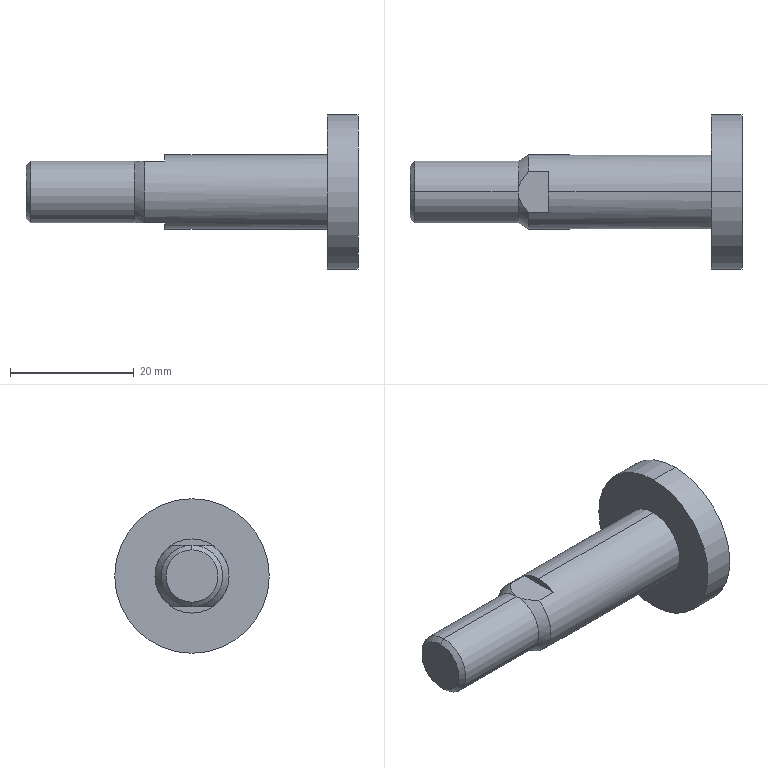Part | SolidWorks | features RefAxis 6, 3DProfileFeature 2, ICE 1, Revolution 1 | 1 solid | 17 faces | box 53.75 x 25 x 25 mm | volume 7288 mm3 | plane 7 | cylinder 6 | cone 4 | commonest cylinder face diameters 10 x2 12 x2 25 x2
STEP:
#1=CARTESIAN_POINT('',(31.25,0.,12.5));
#2=VERTEX_POINT('',#1);
#3=CARTESIAN_POINT('',(31.25,0.,-12.5));
#4=VERTEX_POINT('',#3);
#5=CARTESIAN_POINT('',(31.25,0.,0.));
#6=DIRECTION('',(-1.,0.,0.));
#7=DIRECTION('',(0.,0.,1.));
#8=AXIS2_PLACEMENT_3D('',#5,#6,#7);
#9=CIRCLE('',#8,12.5);
#10=EDGE_CURVE('',#2,#4,#9,.T.);
#11=ORIENTED_EDGE('',*,*,#10,.T.);
#12=CARTESIAN_POINT('',(26.25,0.,-12.5));
#13=VERTEX_POINT('',#12);
#14=CARTESIAN_POINT('',(31.25,0.,-12.5));
#15=DIRECTION('',(-1.,0.,0.));
#16=VECTOR('',#15,1000.);
#17=LINE('',#14,#16);
#18=EDGE_CURVE('',#4,#13,#17,.T.);
#19=ORIENTED_EDGE('',*,*,#18,.T.);
#20=CARTESIAN_POINT('',(26.25,0.,12.5));
#21=VERTEX_POINT('',#20);
#22=CARTESIAN_POINT('',(26.25,0.,0.));
#23=DIRECTION('',(-1.,0.,0.));
#24=DIRECTION('',(0.,0.,1.));
#25=AXIS2_PLACEMENT_3D('',#22,#23,#24);
#26=CIRCLE('',#25,12.5);
#27=EDGE_CURVE('',#21,#13,#26,.T.);
#28=ORIENTED_EDGE('',*,*,#27,.F.);
#29=CARTESIAN_POINT('',(31.25,0.,12.5));
#30=DIRECTION('',(-1.,0.,0.));
#31=VECTOR('',#30,1000.);
#32=LINE('',#29,#31);
#33=EDGE_CURVE('',#2,#21,#32,.T.);
#34=ORIENTED_EDGE('',*,*,#33,.F.);
#35=EDGE_LOOP('',(#11,#19,#28,#34));
#36=FACE_OUTER_BOUND('',#35,.T.);
#37=CARTESIAN_POINT('',(31.25,0.,0.));
#38=DIRECTION('',(-1.,0.,0.));
#39=DIRECTION('',(0.,0.,1.));
#40=AXIS2_PLACEMENT_3D('',#37,#38,#39);
#41=CYLINDRICAL_SURFACE('',#40,12.5);
#42=ADVANCED_FACE('',(#36),#41,.T.);
#43=CARTESIAN_POINT('',(-5.,0.,5.));
#44=VERTEX_POINT('',#43);
#45=CARTESIAN_POINT('',(-5.,0.,-5.));
#46=VERTEX_POINT('',#45);
#47=CARTESIAN_POINT('',(-5.,0.,0.));
#48=DIRECTION('',(-1.,0.,0.));
#49=DIRECTION('',(0.,0.,1.));
#50=AXIS2_PLACEMENT_3D('',#47,#48,#49);
#51=CIRCLE('',#50,5.);
#52=EDGE_CURVE('',#44,#46,#51,.T.);
#53=ORIENTED_EDGE('',*,*,#52,.T.);
#54=CARTESIAN_POINT('',(-21.733,0.,-5.));
#55=VERTEX_POINT('',#54);
#56=CARTESIAN_POINT('',(31.25,0.,-5.));
#57=DIRECTION('',(-1.,0.,0.));
#58=VECTOR('',#57,1000.);
#59=LINE('',#56,#58);
#60=EDGE_CURVE('',#46,#55,#59,.T.);
#61=ORIENTED_EDGE('',*,*,#60,.T.);
#62=CARTESIAN_POINT('',(-21.733,0.,5.));
#63=VERTEX_POINT('',#62);
#64=CARTESIAN_POINT('',(-21.733,0.,0.));
#65=DIRECTION('',(-1.,0.,0.));
#66=DIRECTION('',(0.,0.,1.));
#67=AXIS2_PLACEMENT_3D('',#64,#65,#66);
#68=CIRCLE('',#67,5.);
#69=EDGE_CURVE('',#63,#55,#68,.T.);
#70=ORIENTED_EDGE('',*,*,#69,.F.);
#71=CARTESIAN_POINT('',(31.25,0.,5.));
#72=DIRECTION('',(-1.,0.,0.));
#73=VECTOR('',#72,1000.);
#74=LINE('',#71,#73);
#75=EDGE_CURVE('',#44,#63,#74,.T.);
#76=ORIENTED_EDGE('',*,*,#75,.F.);
#77=EDGE_LOOP('',(#53,#61,#70,#76));
#78=FACE_OUTER_BOUND('',#77,.T.);
#79=CARTESIAN_POINT('',(31.25,0.,0.));
#80=DIRECTION('',(-1.,0.,0.));
#81=DIRECTION('',(0.,0.,1.));
#82=AXIS2_PLACEMENT_3D('',#79,#80,#81);
#83=CYLINDRICAL_SURFACE('',#82,5.);
#84=ADVANCED_FACE('',(#78),#83,.T.);
#85=CARTESIAN_POINT('',(-22.5,0.,4.233));
#86=VERTEX_POINT('',#85);
#87=CARTESIAN_POINT('',(-22.5,0.,-4.233));
#88=VERTEX_POINT('',#87);
#89=CARTESIAN_POINT('',(-22.5,0.,0.));
#90=DIRECTION('',(-1.,0.,0.));
#91=DIRECTION('',(0.,0.,1.));
#92=AXIS2_PLACEMENT_3D('',#89,#90,#91);
#93=CIRCLE('',#92,4.233);
#94=EDGE_CURVE('',#86,#88,#93,.T.);
#95=ORIENTED_EDGE('',*,*,#94,.F.);
#96=CARTESIAN_POINT('',(-21.733,0.,5.));
#97=DIRECTION('',(0.7071,0.,0.7071));
#98=VECTOR('',#97,1000.);
#99=LINE('',#96,#98);
#100=EDGE_CURVE('',#86,#63,#99,.T.);
#101=ORIENTED_EDGE('',*,*,#100,.T.);
#102=ORIENTED_EDGE('',*,*,#69,.T.);
#103=CARTESIAN_POINT('',(-21.733,0.,-5.));
#104=DIRECTION('',(0.7071,0.,-0.7071));
#105=VECTOR('',#104,1000.);
#106=LINE('',#103,#105);
#107=EDGE_CURVE('',#88,#55,#106,.T.);
#108=ORIENTED_EDGE('',*,*,#107,.F.);
#109=EDGE_LOOP('',(#95,#101,#102,#108));
#110=FACE_OUTER_BOUND('',#109,.T.);
#111=CARTESIAN_POINT('',(-21.733,0.,0.));
#112=DIRECTION('',(1.,0.,0.));
#113=DIRECTION('',(0.,0.,-1.));
#114=AXIS2_PLACEMENT_3D('',#111,#112,#113);
#115=CONICAL_SURFACE('',#114,5.,0.7854);
#116=ADVANCED_FACE('',(#110),#115,.T.);
#117=CARTESIAN_POINT('',(26.25,0.,6.));
#118=VERTEX_POINT('',#117);
#119=CARTESIAN_POINT('',(26.25,0.,-6.));
#120=VERTEX_POINT('',#119);
#121=CARTESIAN_POINT('',(26.25,0.,0.));
#122=DIRECTION('',(-1.,0.,0.));
#123=DIRECTION('',(0.,0.,1.));
#124=AXIS2_PLACEMENT_3D('',#121,#122,#123);
#125=CIRCLE('',#124,6.);
#126=EDGE_CURVE('',#118,#120,#125,.T.);
#127=ORIENTED_EDGE('',*,*,#126,.T.);
#128=CARTESIAN_POINT('',(0.,0.,-6.));
#129=VERTEX_POINT('',#128);
#130=CARTESIAN_POINT('',(31.25,0.,-6.));
#131=DIRECTION('',(-1.,0.,0.));
#132=VECTOR('',#131,1000.);
#133=LINE('',#130,#132);
#134=EDGE_CURVE('',#120,#129,#133,.T.);
#135=ORIENTED_EDGE('',*,*,#134,.T.);
#136=CARTESIAN_POINT('',(0.,3.317,-5.));
#137=VERTEX_POINT('',#136);
#138=CARTESIAN_POINT('',(0.,0.,0.));
#139=DIRECTION('',(1.,0.,0.));
#140=DIRECTION('',(0.,0.,-1.));
#141=AXIS2_PLACEMENT_3D('',#138,#139,#140);
#142=CIRCLE('',#141,6.);
#143=EDGE_CURVE('',#129,#137,#142,.T.);
#144=ORIENTED_EDGE('',*,*,#143,.T.);
#145=CARTESIAN_POINT('',(-3.268,3.317,-5.));
#146=VERTEX_POINT('',#145);
#147=CARTESIAN_POINT('',(31.25,3.317,-5.));
#148=DIRECTION('',(1.,0.,0.));
#149=VECTOR('',#148,1000.);
#150=LINE('',#147,#149);
#151=EDGE_CURVE('',#146,#137,#150,.T.);
#152=ORIENTED_EDGE('',*,*,#151,.F.);
#153=CARTESIAN_POINT('',(-3.268,3.317,5.));
#154=VERTEX_POINT('',#153);
#155=CARTESIAN_POINT('',(-3.268,0.,0.));
#156=DIRECTION('',(-1.,0.,0.));
#157=DIRECTION('',(0.,0.,1.));
#158=AXIS2_PLACEMENT_3D('',#155,#156,#157);
#159=CIRCLE('',#158,6.);
#160=EDGE_CURVE('',#154,#146,#159,.T.);
#161=ORIENTED_EDGE('',*,*,#160,.F.);
#162=CARTESIAN_POINT('',(0.,3.317,5.));
#163=VERTEX_POINT('',#162);
#164=CARTESIAN_POINT('',(31.25,3.317,5.));
#165=DIRECTION('',(-1.,0.,0.));
#166=VECTOR('',#165,1000.);
#167=LINE('',#164,#166);
#168=EDGE_CURVE('',#163,#154,#167,.T.);
#169=ORIENTED_EDGE('',*,*,#168,.F.);
#170=CARTESIAN_POINT('',(0.,0.,6.));
#171=VERTEX_POINT('',#170);
#172=CARTESIAN_POINT('',(0.,0.,0.));
#173=DIRECTION('',(1.,0.,0.));
#174=DIRECTION('',(0.,0.,-1.));
#175=AXIS2_PLACEMENT_3D('',#172,#173,#174);
#176=CIRCLE('',#175,6.);
#177=EDGE_CURVE('',#163,#171,#176,.T.);
#178=ORIENTED_EDGE('',*,*,#177,.T.);
#179=CARTESIAN_POINT('',(31.25,0.,6.));
#180=DIRECTION('',(-1.,0.,0.));
#181=VECTOR('',#180,1000.);
#182=LINE('',#179,#181);
#183=EDGE_CURVE('',#118,#171,#182,.T.);
#184=ORIENTED_EDGE('',*,*,#183,.F.);
#185=EDGE_LOOP('',(#127,#135,#144,#152,#161,#169,#178,#184));
#186=FACE_OUTER_BOUND('',#185,.T.);
#187=CARTESIAN_POINT('',(31.25,0.,0.));
#188=DIRECTION('',(-1.,0.,0.));
#189=DIRECTION('',(0.,0.,1.));
#190=AXIS2_PLACEMENT_3D('',#187,#188,#189);
#191=CYLINDRICAL_SURFACE('',#190,6.);
#192=ADVANCED_FACE('',(#186),#191,.T.);
#193=CARTESIAN_POINT('',(-3.268,3.317,5.));
#194=CARTESIAN_POINT('',(-3.488,3.087,5.));
#195=CARTESIAN_POINT('',(-3.699,2.85,5.));
#196=CARTESIAN_POINT('',(-4.096,2.354,5.));
#197=CARTESIAN_POINT('',(-4.281,2.095,5.));
#198=CARTESIAN_POINT('',(-4.609,1.542,5.));
#199=CARTESIAN_POINT('',(-4.748,1.251,5.));
#200=CARTESIAN_POINT('',(-4.944,0.642,5.));
#201=CARTESIAN_POINT('',(-5.,0.3184,5.));
#202=CARTESIAN_POINT('',(-5.,0.,5.));
#203=B_SPLINE_CURVE_WITH_KNOTS('',3,(#193,#194,#195,#196,#197,#198,#199,#200,#201,#202),.UNSPECIFIED.,.F.,.F.,(4,2,2,2,4),(0.01312,0.01407,0.01502,0.01598,0.01693),.UNSPECIFIED.);
#204=EDGE_CURVE('',#154,#44,#203,.T.);
#205=ORIENTED_EDGE('',*,*,#204,.F.);
#206=ORIENTED_EDGE('',*,*,#160,.T.);
#207=CARTESIAN_POINT('',(-5.,0.,-5.));
#208=CARTESIAN_POINT('',(-5.,0.3184,-5.));
#209=CARTESIAN_POINT('',(-4.944,0.642,-5.));
#210=CARTESIAN_POINT('',(-4.748,1.251,-5.));
#211=CARTESIAN_POINT('',(-4.609,1.542,-5.));
#212=CARTESIAN_POINT('',(-4.281,2.095,-5.));
#213=CARTESIAN_POINT('',(-4.096,2.354,-5.));
#214=CARTESIAN_POINT('',(-3.699,2.85,-5.));
#215=CARTESIAN_POINT('',(-3.488,3.087,-5.));
#216=CARTESIAN_POINT('',(-3.268,3.317,-5.));
#217=B_SPLINE_CURVE_WITH_KNOTS('',3,(#207,#208,#209,#210,#211,#212,#213,#214,#215,#216),.UNSPECIFIED.,.F.,.F.,(4,2,2,2,4),(0.01206,0.01301,0.01397,0.01492,0.01587),.UNSPECIFIED.);
#218=EDGE_CURVE('',#46,#146,#217,.T.);
#219=ORIENTED_EDGE('',*,*,#218,.F.);
#220=ORIENTED_EDGE('',*,*,#52,.F.);
#221=EDGE_LOOP('',(#205,#206,#219,#220));
#222=FACE_OUTER_BOUND('',#221,.T.);
#223=CARTESIAN_POINT('',(-3.268,0.,0.));
#224=DIRECTION('',(1.,0.,0.));
#225=DIRECTION('',(0.,0.,-1.));
#226=AXIS2_PLACEMENT_3D('',#223,#224,#225);
#227=CONICAL_SURFACE('',#226,6.,0.5236);
#228=ADVANCED_FACE('',(#222),#227,.T.);
#229=CARTESIAN_POINT('',(-3.268,-3.317,5.));
#230=VERTEX_POINT('',#229);
#231=CARTESIAN_POINT('',(-5.,0.,5.));
#232=CARTESIAN_POINT('',(-5.,-0.1588,5.));
#233=CARTESIAN_POINT('',(-4.987,-0.3175,5.));
#234=CARTESIAN_POINT('',(-4.935,-0.6349,5.));
#235=CARTESIAN_POINT('',(-4.896,-0.7921,5.));
#236=CARTESIAN_POINT('',(-4.749,-1.249,5.));
#237=CARTESIAN_POINT('',(-4.609,-1.54,5.));
#238=CARTESIAN_POINT('',(-4.283,-2.092,5.));
#239=CARTESIAN_POINT('',(-4.098,-2.351,5.));
#240=CARTESIAN_POINT('',(-3.701,-2.848,5.));
#241=CARTESIAN_POINT('',(-3.489,-3.086,5.));
#242=CARTESIAN_POINT('',(-3.268,-3.317,5.));
#243=B_SPLINE_CURVE_WITH_KNOTS('',3,(#231,#232,#233,#234,#235,#236,#237,#238,#239,#240,#241,#242),.UNSPECIFIED.,.F.,.F.,(4,2,2,2,2,4),(0.01693,0.0174,0.01787,0.01882,0.01977,0.02072),.UNSPECIFIED.);
#244=EDGE_CURVE('',#44,#230,#243,.T.);
#245=ORIENTED_EDGE('',*,*,#244,.F.);
#246=CARTESIAN_POINT('',(-5.,0.,0.));
#247=DIRECTION('',(-1.,0.,0.));
#248=DIRECTION('',(0.,0.,1.));
#249=AXIS2_PLACEMENT_3D('',#246,#247,#248);
#250=CIRCLE('',#249,5.);
#251=EDGE_CURVE('',#46,#44,#250,.T.);
#252=ORIENTED_EDGE('',*,*,#251,.F.);
#253=CARTESIAN_POINT('',(-3.268,-3.317,-5.));
#254=VERTEX_POINT('',#253);
#255=CARTESIAN_POINT('',(-3.268,-3.317,-5.));
#256=CARTESIAN_POINT('',(-3.489,-3.086,-5.));
#257=CARTESIAN_POINT('',(-3.701,-2.848,-5.));
#258=CARTESIAN_POINT('',(-4.098,-2.351,-5.));
#259=CARTESIAN_POINT('',(-4.283,-2.092,-5.));
#260=CARTESIAN_POINT('',(-4.609,-1.54,-5.));
#261=CARTESIAN_POINT('',(-4.749,-1.249,-5.));
#262=CARTESIAN_POINT('',(-4.896,-0.7921,-5.));
#263=CARTESIAN_POINT('',(-4.935,-0.6349,-5.));
#264=CARTESIAN_POINT('',(-4.987,-0.3175,-5.));
#265=CARTESIAN_POINT('',(-5.,-0.1588,-5.));
#266=CARTESIAN_POINT('',(-5.,0.,-5.));
#267=B_SPLINE_CURVE_WITH_KNOTS('',3,(#255,#256,#257,#258,#259,#260,#261,#262,#263,#264,#265,#266),.UNSPECIFIED.,.F.,.F.,(4,2,2,2,2,4),(0.008255,0.009206,0.01016,0.01111,0.01158,0.01206),.UNSPECIFIED.);
#268=EDGE_CURVE('',#254,#46,#267,.T.);
#269=ORIENTED_EDGE('',*,*,#268,.F.);
#270=CARTESIAN_POINT('',(-3.268,0.,0.));
#271=DIRECTION('',(-1.,0.,0.));
#272=DIRECTION('',(0.,0.,1.));
#273=AXIS2_PLACEMENT_3D('',#270,#271,#272);
#274=CIRCLE('',#273,6.);
#275=EDGE_CURVE('',#254,#230,#274,.T.);
#276=ORIENTED_EDGE('',*,*,#275,.T.);
#277=EDGE_LOOP('',(#245,#252,#269,#276));
#278=FACE_OUTER_BOUND('',#277,.T.);
#279=CARTESIAN_POINT('',(-3.268,0.,0.));
#280=DIRECTION('',(1.,0.,0.));
#281=DIRECTION('',(0.,0.,-1.));
#282=AXIS2_PLACEMENT_3D('',#279,#280,#281);
#283=CONICAL_SURFACE('',#282,6.,0.5236);
#284=ADVANCED_FACE('',(#278),#283,.T.);
#285=ORIENTED_EDGE('',*,*,#134,.F.);
#286=CARTESIAN_POINT('',(26.25,0.,0.));
#287=DIRECTION('',(-1.,0.,0.));
#288=DIRECTION('',(0.,0.,1.));
#289=AXIS2_PLACEMENT_3D('',#286,#287,#288);
#290=CIRCLE('',#289,6.);
#291=EDGE_CURVE('',#120,#118,#290,.T.);
#292=ORIENTED_EDGE('',*,*,#291,.T.);
#293=ORIENTED_EDGE('',*,*,#183,.T.);
#294=CARTESIAN_POINT('',(0.,-3.317,5.));
#295=VERTEX_POINT('',#294);
#296=CARTESIAN_POINT('',(0.,0.,0.));
#297=DIRECTION('',(1.,0.,0.));
#298=DIRECTION('',(0.,0.,-1.));
#299=AXIS2_PLACEMENT_3D('',#296,#297,#298);
#300=CIRCLE('',#299,6.);
#301=EDGE_CURVE('',#171,#295,#300,.T.);
#302=ORIENTED_EDGE('',*,*,#301,.T.);
#303=CARTESIAN_POINT('',(31.25,-3.317,5.));
#304=DIRECTION('',(1.,0.,0.));
#305=VECTOR('',#304,1000.);
#306=LINE('',#303,#305);
#307=EDGE_CURVE('',#230,#295,#306,.T.);
#308=ORIENTED_EDGE('',*,*,#307,.F.);
#309=ORIENTED_EDGE('',*,*,#275,.F.);
#310=CARTESIAN_POINT('',(0.,-3.317,-5.));
#311=VERTEX_POINT('',#310);
#312=CARTESIAN_POINT('',(31.25,-3.317,-5.));
#313=DIRECTION('',(-1.,0.,0.));
#314=VECTOR('',#313,1000.);
#315=LINE('',#312,#314);
#316=EDGE_CURVE('',#311,#254,#315,.T.);
#317=ORIENTED_EDGE('',*,*,#316,.F.);
#318=CARTESIAN_POINT('',(0.,0.,0.));
#319=DIRECTION('',(1.,0.,0.));
#320=DIRECTION('',(0.,0.,-1.));
#321=AXIS2_PLACEMENT_3D('',#318,#319,#320);
#322=CIRCLE('',#321,6.);
#323=EDGE_CURVE('',#311,#129,#322,.T.);
#324=ORIENTED_EDGE('',*,*,#323,.T.);
#325=EDGE_LOOP('',(#285,#292,#293,#302,#308,#309,#317,#324));
#326=FACE_OUTER_BOUND('',#325,.T.);
#327=CARTESIAN_POINT('',(31.25,0.,0.));
#328=DIRECTION('',(-1.,0.,0.));
#329=DIRECTION('',(0.,0.,1.));
#330=AXIS2_PLACEMENT_3D('',#327,#328,#329);
#331=CYLINDRICAL_SURFACE('',#330,6.);
#332=ADVANCED_FACE('',(#326),#331,.T.);
#333=CARTESIAN_POINT('',(-22.5,0.,0.));
#334=DIRECTION('',(-1.,0.,0.));
#335=DIRECTION('',(0.,0.,1.));
#336=AXIS2_PLACEMENT_3D('',#333,#334,#335);
#337=CIRCLE('',#336,4.233);
#338=EDGE_CURVE('',#88,#86,#337,.T.);
#339=ORIENTED_EDGE('',*,*,#338,.T.);
#340=ORIENTED_EDGE('',*,*,#94,.T.);
#341=EDGE_LOOP('',(#339,#340));
#342=FACE_OUTER_BOUND('',#341,.T.);
#343=CARTESIAN_POINT('',(-22.5,0.,0.));
#344=DIRECTION('',(1.,0.,0.));
#345=DIRECTION('',(0.,0.,-1.));
#346=AXIS2_PLACEMENT_3D('',#343,#344,#345);
#347=PLANE('',#346);
#348=ADVANCED_FACE('',(#342),#347,.F.);
#349=ORIENTED_EDGE('',*,*,#100,.F.);
#350=ORIENTED_EDGE('',*,*,#338,.F.);
#351=ORIENTED_EDGE('',*,*,#107,.T.);
#352=CARTESIAN_POINT('',(-21.733,0.,0.));
#353=DIRECTION('',(-1.,0.,0.));
#354=DIRECTION('',(0.,0.,1.));
#355=AXIS2_PLACEMENT_3D('',#352,#353,#354);
#356=CIRCLE('',#355,5.);
#357=EDGE_CURVE('',#55,#63,#356,.T.);
#358=ORIENTED_EDGE('',*,*,#357,.T.);
#359=EDGE_LOOP('',(#349,#350,#351,#358));
#360=FACE_OUTER_BOUND('',#359,.T.);
#361=CARTESIAN_POINT('',(-21.733,0.,0.));
#362=DIRECTION('',(1.,0.,0.));
#363=DIRECTION('',(0.,0.,-1.));
#364=AXIS2_PLACEMENT_3D('',#361,#362,#363);
#365=CONICAL_SURFACE('',#364,5.,0.7854);
#366=ADVANCED_FACE('',(#360),#365,.T.);
#367=ORIENTED_EDGE('',*,*,#60,.F.);
#368=ORIENTED_EDGE('',*,*,#251,.T.);
#369=ORIENTED_EDGE('',*,*,#75,.T.);
#370=ORIENTED_EDGE('',*,*,#357,.F.);
#371=EDGE_LOOP('',(#367,#368,#369,#370));
#372=FACE_OUTER_BOUND('',#371,.T.);
#373=CARTESIAN_POINT('',(31.25,0.,0.));
#374=DIRECTION('',(-1.,0.,0.));
#375=DIRECTION('',(0.,0.,1.));
#376=AXIS2_PLACEMENT_3D('',#373,#374,#375);
#377=CYLINDRICAL_SURFACE('',#376,5.);
#378=ADVANCED_FACE('',(#372),#377,.T.);
#379=ORIENTED_EDGE('',*,*,#126,.F.);
#380=ORIENTED_EDGE('',*,*,#291,.F.);
#381=EDGE_LOOP('',(#379,#380));
#382=FACE_BOUND('',#381,.T.);
#383=ORIENTED_EDGE('',*,*,#27,.T.);
#384=CARTESIAN_POINT('',(26.25,0.,0.));
#385=DIRECTION('',(-1.,0.,0.));
#386=DIRECTION('',(0.,0.,1.));
#387=AXIS2_PLACEMENT_3D('',#384,#385,#386);
#388=CIRCLE('',#387,12.5);
#389=EDGE_CURVE('',#13,#21,#388,.T.);
#390=ORIENTED_EDGE('',*,*,#389,.T.);
#391=EDGE_LOOP('',(#383,#390));
#392=FACE_OUTER_BOUND('',#391,.T.);
#393=CARTESIAN_POINT('',(26.25,6.,0.));
#394=DIRECTION('',(1.,0.,0.));
#395=DIRECTION('',(0.,0.,-1.));
#396=AXIS2_PLACEMENT_3D('',#393,#394,#395);
#397=PLANE('',#396);
#398=ADVANCED_FACE('',(#382,#392),#397,.F.);
#399=ORIENTED_EDGE('',*,*,#18,.F.);
#400=CARTESIAN_POINT('',(31.25,0.,0.));
#401=DIRECTION('',(-1.,0.,0.));
#402=DIRECTION('',(0.,0.,1.));
#403=AXIS2_PLACEMENT_3D('',#400,#401,#402);
#404=CIRCLE('',#403,12.5);
#405=EDGE_CURVE('',#4,#2,#404,.T.);
#406=ORIENTED_EDGE('',*,*,#405,.T.);
#407=ORIENTED_EDGE('',*,*,#33,.T.);
#408=ORIENTED_EDGE('',*,*,#389,.F.);
#409=EDGE_LOOP('',(#399,#406,#407,#408));
#410=FACE_OUTER_BOUND('',#409,.T.);
#411=CARTESIAN_POINT('',(31.25,0.,0.));
#412=DIRECTION('',(-1.,0.,0.));
#413=DIRECTION('',(0.,0.,1.));
#414=AXIS2_PLACEMENT_3D('',#411,#412,#413);
#415=CYLINDRICAL_SURFACE('',#414,12.5);
#416=ADVANCED_FACE('',(#410),#415,.T.);
#417=ORIENTED_EDGE('',*,*,#10,.F.);
#418=ORIENTED_EDGE('',*,*,#405,.F.);
#419=EDGE_LOOP('',(#417,#418));
#420=FACE_OUTER_BOUND('',#419,.T.);
#421=CARTESIAN_POINT('',(31.25,12.5,0.));
#422=DIRECTION('',(-1.,0.,0.));
#423=DIRECTION('',(0.,0.,1.));
#424=AXIS2_PLACEMENT_3D('',#421,#422,#423);
#425=PLANE('',#424);
#426=ADVANCED_FACE('',(#420),#425,.F.);
#427=ORIENTED_EDGE('',*,*,#316,.T.);
#428=ORIENTED_EDGE('',*,*,#268,.T.);
#429=ORIENTED_EDGE('',*,*,#218,.T.);
#430=ORIENTED_EDGE('',*,*,#151,.T.);
#431=CARTESIAN_POINT('',(0.,-7.,-5.));
#432=DIRECTION('',(0.,1.,0.));
#433=VECTOR('',#432,1000.);
#434=LINE('',#431,#433);
#435=EDGE_CURVE('',#311,#137,#434,.T.);
#436=ORIENTED_EDGE('',*,*,#435,.F.);
#437=EDGE_LOOP('',(#427,#428,#429,#430,#436));
#438=FACE_OUTER_BOUND('',#437,.T.);
#439=CARTESIAN_POINT('',(-5.,-7.,-5.));
#440=DIRECTION('',(0.,0.,-1.));
#441=DIRECTION('',(-1.,0.,0.));
#442=AXIS2_PLACEMENT_3D('',#439,#440,#441);
#443=PLANE('',#442);
#444=ADVANCED_FACE('',(#438),#443,.T.);
#445=ORIENTED_EDGE('',*,*,#435,.T.);
#446=ORIENTED_EDGE('',*,*,#143,.F.);
#447=ORIENTED_EDGE('',*,*,#323,.F.);
#448=EDGE_LOOP('',(#445,#446,#447));
#449=FACE_OUTER_BOUND('',#448,.T.);
#450=CARTESIAN_POINT('',(0.,0.,0.));
#451=DIRECTION('',(1.,0.,0.));
#452=DIRECTION('',(0.,0.,-1.));
#453=AXIS2_PLACEMENT_3D('',#450,#451,#452);
#454=PLANE('',#453);
#455=ADVANCED_FACE('',(#449),#454,.F.);
#456=CARTESIAN_POINT('',(0.,7.,5.));
#457=DIRECTION('',(0.,-1.,0.));
#458=VECTOR('',#457,1000.);
#459=LINE('',#456,#458);
#460=EDGE_CURVE('',#163,#295,#459,.T.);
#461=ORIENTED_EDGE('',*,*,#460,.T.);
#462=ORIENTED_EDGE('',*,*,#301,.F.);
#463=ORIENTED_EDGE('',*,*,#177,.F.);
#464=EDGE_LOOP('',(#461,#462,#463));
#465=FACE_OUTER_BOUND('',#464,.T.);
#466=CARTESIAN_POINT('',(0.,0.,0.));
#467=DIRECTION('',(1.,0.,0.));
#468=DIRECTION('',(0.,0.,-1.));
#469=AXIS2_PLACEMENT_3D('',#466,#467,#468);
#470=PLANE('',#469);
#471=ADVANCED_FACE('',(#465),#470,.F.);
#472=ORIENTED_EDGE('',*,*,#168,.T.);
#473=ORIENTED_EDGE('',*,*,#204,.T.);
#474=ORIENTED_EDGE('',*,*,#244,.T.);
#475=ORIENTED_EDGE('',*,*,#307,.T.);
#476=ORIENTED_EDGE('',*,*,#460,.F.);
#477=EDGE_LOOP('',(#472,#473,#474,#475,#476));
#478=FACE_OUTER_BOUND('',#477,.T.);
#479=CARTESIAN_POINT('',(-5.,7.,5.));
#480=DIRECTION('',(0.,0.,1.));
#481=DIRECTION('',(1.,0.,0.));
#482=AXIS2_PLACEMENT_3D('',#479,#480,#481);
#483=PLANE('',#482);
#484=ADVANCED_FACE('',(#478),#483,.T.);
#485=CLOSED_SHELL('',(#42,#84,#116,#192,#228,#284,#332,#348,#366,#378,#398,#416,#426,#444,#455,#471,#484));
#486=MANIFOLD_SOLID_BREP('',#485);
#487=CARTESIAN_POINT('',(0.,0.,0.));
#488=DIRECTION('',(0.,0.,1.));
#489=DIRECTION('',(1.,0.,0.));
#490=AXIS2_PLACEMENT_3D('',#487,#488,#489);
#491=(LENGTH_UNIT()NAMED_UNIT(*)SI_UNIT(.MILLI.,.METRE.));
#492=UNCERTAINTY_MEASURE_WITH_UNIT(LENGTH_MEASURE(0.00001),#491,'','');
#493=(NAMED_UNIT(*)PLANE_ANGLE_UNIT()SI_UNIT($,.RADIAN.));
#494=(NAMED_UNIT(*)SI_UNIT($,.STERADIAN.)SOLID_ANGLE_UNIT());
#495=(GEOMETRIC_REPRESENTATION_CONTEXT(3)GLOBAL_UNCERTAINTY_ASSIGNED_CONTEXT((#492))GLOBAL_UNIT_ASSIGNED_CONTEXT((#491,#493,#494))REPRESENTATION_CONTEXT('',''));
#496=ADVANCED_BREP_SHAPE_REPRESENTATION('',(#486,#490),#495);